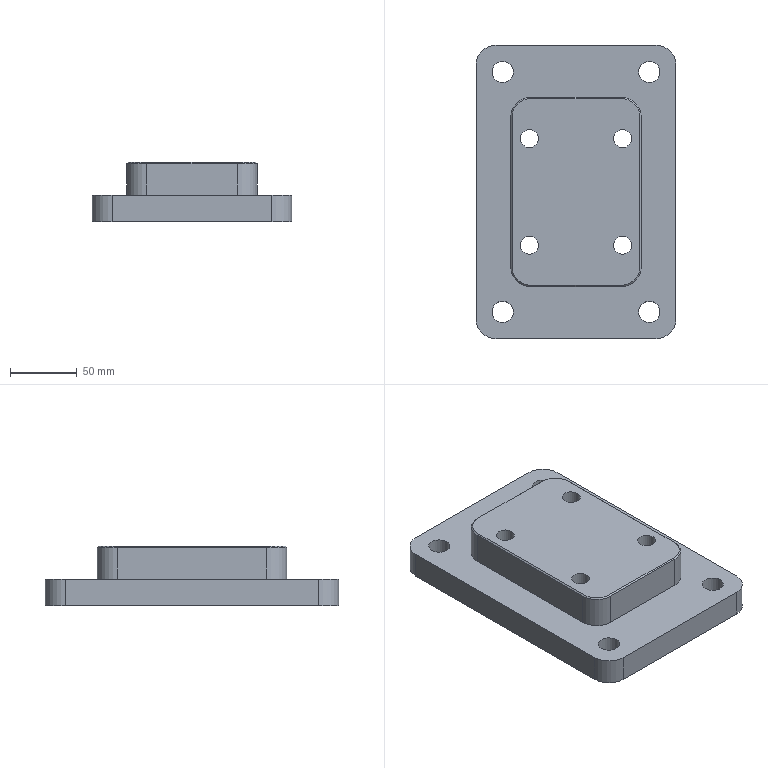NC program | NX | posted with a generic post | part box 150 x 220 x 45 mm
Lines 1 to 39 of 5916:
N10 G17 G21 G94 G90
(DRILLING , TOOL : ZXZ)
N12 T01 M6
N14 G54
N16 G17 G0 G90 X90. Y-55. S5000 M3
N18 G43 Z30. H1
N20 G94 G81 G98 Z-1. F250. R3.
N22 X40. Y-35.
N24 X-40.
N26 X-90. Y-55.
N28 Y55.
N30 X-40. Y35.
N32 X40.
N34 X90. Y55.
N36 G80
N38 G0 X90. Y55. Z30.
N40 M5
(DRILLING_COPY , TOOL : 13.5ZT)
N42 T13 M6
N44 G54
N46 G17 G0 G90 X90. Y-55. S2000 M3
N48 G43 Z30. H13
N50 G94 G83 G98 Z-25.556 F200. Q2. R3.
N52 X40. Y-35. Z-50.556
N54 X-40.
N56 X-90. Y-55. Z-25.556
N58 Y55.
N60 X-40. Y35. Z-50.556
N62 X40.
N64 X90. Y55. Z-25.556
N66 G80
N68 G0 X90. Y55. Z30.
N70 M5